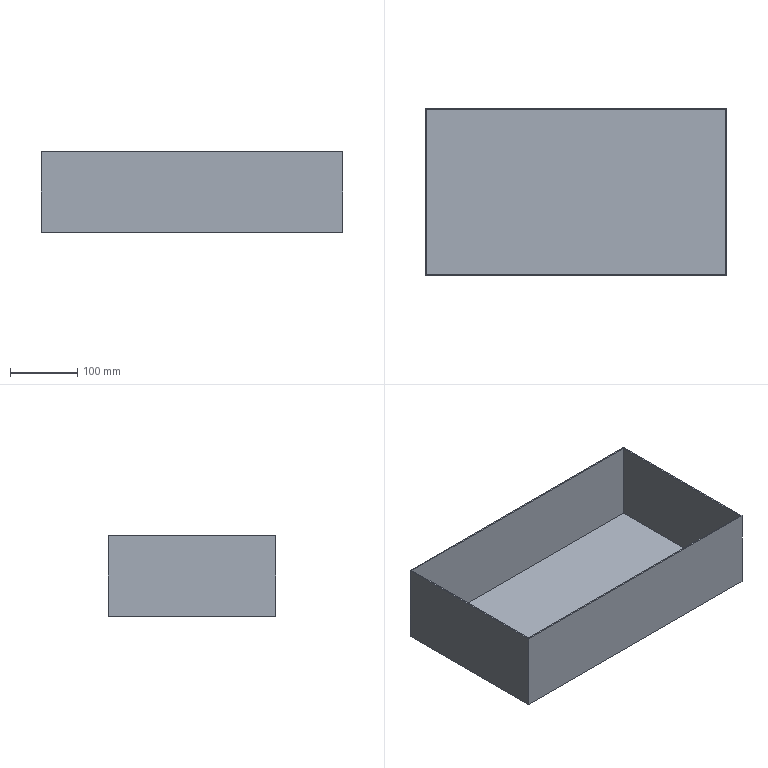Part | STEP file | NG parts material box | 1 solid | 11 faces | box 450 x 250 x 120 mm | volume 553512 mm3 | plane 11
STEP:
#1=CARTESIAN_POINT('',(0.,0.,0.));
#2=DIRECTION('',(0.,0.,1.));
#3=DIRECTION('',(1.,0.,0.));
#4=AXIS2_PLACEMENT_3D('',#1,#2,#3);
#5=CARTESIAN_POINT('',(-225.,-125.,0.));
#6=VERTEX_POINT('',#5);
#7=CARTESIAN_POINT('',(225.,-125.,0.));
#8=VERTEX_POINT('',#7);
#9=CARTESIAN_POINT('',(225.,-125.,0.));
#10=DIRECTION('',(1.,0.,0.));
#11=VECTOR('',#10,1.);
#12=LINE('',#9,#11);
#13=CARTESIAN_POINT('',(225.,-125.,0.));
#14=DIRECTION('',(0.,0.,1.));
#15=DIRECTION('',(1.,0.,0.));
#16=AXIS2_PLACEMENT_3D('',#13,#14,#15);
#17=PLANE('',#16);
#18=CARTESIAN_POINT('',(0.,0.));
#19=DIRECTION('',(1.,0.));
#20=VECTOR('',#19,1.);
#21=LINE('',#18,#20);
#22=(GEOMETRIC_REPRESENTATION_CONTEXT(2)PARAMETRIC_REPRESENTATION_CONTEXT()REPRESENTATION_CONTEXT('',''));
#23=DEFINITIONAL_REPRESENTATION('',(#21),#22);
#24=PCURVE('',#17,#23);
#25=CARTESIAN_POINT('',(-225.,-125.,120.));
#26=DIRECTION('',(0.,1.,0.));
#27=DIRECTION('',(0.,0.,1.));
#28=AXIS2_PLACEMENT_3D('',#25,#26,#27);
#29=PLANE('',#28);
#30=CARTESIAN_POINT('',(-120.,450.));
#31=DIRECTION('',(0.,1.));
#32=VECTOR('',#31,1.);
#33=LINE('',#30,#32);
#34=(GEOMETRIC_REPRESENTATION_CONTEXT(2)PARAMETRIC_REPRESENTATION_CONTEXT()REPRESENTATION_CONTEXT('',''));
#35=DEFINITIONAL_REPRESENTATION('',(#33),#34);
#36=PCURVE('',#29,#35);
#37=SURFACE_CURVE('',#12,(#24,#36),.PCURVE_S1.);
#38=EDGE_CURVE('',#6,#8,#37,.T.);
#39=ORIENTED_EDGE('',*,*,#38,.F.);
#40=CARTESIAN_POINT('',(-225.,125.,0.));
#41=VERTEX_POINT('',#40);
#42=CARTESIAN_POINT('',(-225.,-125.,0.));
#43=DIRECTION('',(0.,-1.,0.));
#44=VECTOR('',#43,1.);
#45=LINE('',#42,#44);
#46=CARTESIAN_POINT('',(-450.,0.));
#47=DIRECTION('',(0.,-1.));
#48=VECTOR('',#47,1.);
#49=LINE('',#46,#48);
#50=(GEOMETRIC_REPRESENTATION_CONTEXT(2)PARAMETRIC_REPRESENTATION_CONTEXT()REPRESENTATION_CONTEXT('',''));
#51=DEFINITIONAL_REPRESENTATION('',(#49),#50);
#52=PCURVE('',#17,#51);
#53=CARTESIAN_POINT('',(-225.,125.,120.));
#54=DIRECTION('',(1.,0.,0.));
#55=DIRECTION('',(0.,1.,0.));
#56=AXIS2_PLACEMENT_3D('',#53,#54,#55);
#57=PLANE('',#56);
#58=CARTESIAN_POINT('',(-250.,-120.));
#59=DIRECTION('',(-1.,0.));
#60=VECTOR('',#59,1.);
#61=LINE('',#58,#60);
#62=(GEOMETRIC_REPRESENTATION_CONTEXT(2)PARAMETRIC_REPRESENTATION_CONTEXT()REPRESENTATION_CONTEXT('',''));
#63=DEFINITIONAL_REPRESENTATION('',(#61),#62);
#64=PCURVE('',#57,#63);
#65=SURFACE_CURVE('',#45,(#52,#64),.PCURVE_S1.);
#66=EDGE_CURVE('',#41,#6,#65,.T.);
#67=ORIENTED_EDGE('',*,*,#66,.F.);
#68=CARTESIAN_POINT('',(225.,125.,0.));
#69=VERTEX_POINT('',#68);
#70=CARTESIAN_POINT('',(225.,125.,0.));
#71=DIRECTION('',(-1.,0.,0.));
#72=VECTOR('',#71,1.);
#73=LINE('',#70,#72);
#74=CARTESIAN_POINT('',(0.,250.));
#75=DIRECTION('',(-1.,0.));
#76=VECTOR('',#75,1.);
#77=LINE('',#74,#76);
#78=(GEOMETRIC_REPRESENTATION_CONTEXT(2)PARAMETRIC_REPRESENTATION_CONTEXT()REPRESENTATION_CONTEXT('',''));
#79=DEFINITIONAL_REPRESENTATION('',(#77),#78);
#80=PCURVE('',#17,#79);
#81=CARTESIAN_POINT('',(-225.,125.,120.));
#82=DIRECTION('',(0.,-1.,0.));
#83=DIRECTION('',(0.,0.,-1.));
#84=AXIS2_PLACEMENT_3D('',#81,#82,#83);
#85=PLANE('',#84);
#86=CARTESIAN_POINT('',(120.,450.));
#87=DIRECTION('',(0.,-1.));
#88=VECTOR('',#87,1.);
#89=LINE('',#86,#88);
#90=(GEOMETRIC_REPRESENTATION_CONTEXT(2)PARAMETRIC_REPRESENTATION_CONTEXT()REPRESENTATION_CONTEXT('',''));
#91=DEFINITIONAL_REPRESENTATION('',(#89),#90);
#92=PCURVE('',#85,#91);
#93=SURFACE_CURVE('',#73,(#80,#92),.PCURVE_S1.);
#94=EDGE_CURVE('',#69,#41,#93,.T.);
#95=ORIENTED_EDGE('',*,*,#94,.F.);
#96=CARTESIAN_POINT('',(225.,-125.,0.));
#97=DIRECTION('',(0.,1.,0.));
#98=VECTOR('',#97,1.);
#99=LINE('',#96,#98);
#100=CARTESIAN_POINT('',(0.,0.));
#101=DIRECTION('',(0.,1.));
#102=VECTOR('',#101,1.);
#103=LINE('',#100,#102);
#104=(GEOMETRIC_REPRESENTATION_CONTEXT(2)PARAMETRIC_REPRESENTATION_CONTEXT()REPRESENTATION_CONTEXT('',''));
#105=DEFINITIONAL_REPRESENTATION('',(#103),#104);
#106=PCURVE('',#17,#105);
#107=CARTESIAN_POINT('',(225.,125.,120.));
#108=DIRECTION('',(-1.,0.,0.));
#109=DIRECTION('',(0.,-1.,0.));
#110=AXIS2_PLACEMENT_3D('',#107,#108,#109);
#111=PLANE('',#110);
#112=CARTESIAN_POINT('',(250.,-120.));
#113=DIRECTION('',(-1.,0.));
#114=VECTOR('',#113,1.);
#115=LINE('',#112,#114);
#116=(GEOMETRIC_REPRESENTATION_CONTEXT(2)PARAMETRIC_REPRESENTATION_CONTEXT()REPRESENTATION_CONTEXT('',''));
#117=DEFINITIONAL_REPRESENTATION('',(#115),#116);
#118=PCURVE('',#111,#117);
#119=SURFACE_CURVE('',#99,(#106,#118),.PCURVE_S1.);
#120=EDGE_CURVE('',#8,#69,#119,.T.);
#121=ORIENTED_EDGE('',*,*,#120,.F.);
#122=EDGE_LOOP('',(#39,#67,#95,#121));
#123=FACE_BOUND('',#122,.T.);
#124=ADVANCED_FACE('',(#123),#17,.F.);
#125=CARTESIAN_POINT('',(225.,125.,120.));
#126=VERTEX_POINT('',#125);
#127=CARTESIAN_POINT('',(225.,125.,120.));
#128=DIRECTION('',(0.,0.,-1.));
#129=VECTOR('',#128,1.);
#130=LINE('',#127,#129);
#131=CARTESIAN_POINT('',(0.,0.));
#132=DIRECTION('',(0.,-1.));
#133=VECTOR('',#132,1.);
#134=LINE('',#131,#133);
#135=(GEOMETRIC_REPRESENTATION_CONTEXT(2)PARAMETRIC_REPRESENTATION_CONTEXT()REPRESENTATION_CONTEXT('',''));
#136=DEFINITIONAL_REPRESENTATION('',(#134),#135);
#137=PCURVE('',#111,#136);
#138=CARTESIAN_POINT('',(0.,450.));
#139=DIRECTION('',(1.,0.));
#140=VECTOR('',#139,1.);
#141=LINE('',#138,#140);
#142=(GEOMETRIC_REPRESENTATION_CONTEXT(2)PARAMETRIC_REPRESENTATION_CONTEXT()REPRESENTATION_CONTEXT('',''));
#143=DEFINITIONAL_REPRESENTATION('',(#141),#142);
#144=PCURVE('',#85,#143);
#145=SURFACE_CURVE('',#130,(#137,#144),.PCURVE_S1.);
#146=EDGE_CURVE('',#126,#69,#145,.T.);
#147=ORIENTED_EDGE('',*,*,#146,.F.);
#148=CARTESIAN_POINT('',(225.,-125.,120.));
#149=VERTEX_POINT('',#148);
#150=CARTESIAN_POINT('',(225.,125.,120.));
#151=DIRECTION('',(0.,1.,0.));
#152=VECTOR('',#151,1.);
#153=LINE('',#150,#152);
#154=CARTESIAN_POINT('',(0.,0.));
#155=DIRECTION('',(-1.,0.));
#156=VECTOR('',#155,1.);
#157=LINE('',#154,#156);
#158=(GEOMETRIC_REPRESENTATION_CONTEXT(2)PARAMETRIC_REPRESENTATION_CONTEXT()REPRESENTATION_CONTEXT('',''));
#159=DEFINITIONAL_REPRESENTATION('',(#157),#158);
#160=PCURVE('',#111,#159);
#161=CARTESIAN_POINT('',(225.,-125.,120.));
#162=DIRECTION('',(0.,0.,1.));
#163=DIRECTION('',(1.,0.,0.));
#164=AXIS2_PLACEMENT_3D('',#161,#162,#163);
#165=PLANE('',#164);
#166=CARTESIAN_POINT('',(0.,250.));
#167=DIRECTION('',(0.,1.));
#168=VECTOR('',#167,1.);
#169=LINE('',#166,#168);
#170=(GEOMETRIC_REPRESENTATION_CONTEXT(2)PARAMETRIC_REPRESENTATION_CONTEXT()REPRESENTATION_CONTEXT('',''));
#171=DEFINITIONAL_REPRESENTATION('',(#169),#170);
#172=PCURVE('',#165,#171);
#173=SURFACE_CURVE('',#153,(#160,#172),.PCURVE_S1.);
#174=EDGE_CURVE('',#149,#126,#173,.T.);
#175=ORIENTED_EDGE('',*,*,#174,.F.);
#176=CARTESIAN_POINT('',(225.,-125.,120.));
#177=DIRECTION('',(0.,0.,1.));
#178=VECTOR('',#177,1.);
#179=LINE('',#176,#178);
#180=CARTESIAN_POINT('',(250.,0.));
#181=DIRECTION('',(0.,1.));
#182=VECTOR('',#181,1.);
#183=LINE('',#180,#182);
#184=(GEOMETRIC_REPRESENTATION_CONTEXT(2)PARAMETRIC_REPRESENTATION_CONTEXT()REPRESENTATION_CONTEXT('',''));
#185=DEFINITIONAL_REPRESENTATION('',(#183),#184);
#186=PCURVE('',#111,#185);
#187=CARTESIAN_POINT('',(0.,450.));
#188=DIRECTION('',(1.,0.));
#189=VECTOR('',#188,1.);
#190=LINE('',#187,#189);
#191=(GEOMETRIC_REPRESENTATION_CONTEXT(2)PARAMETRIC_REPRESENTATION_CONTEXT()REPRESENTATION_CONTEXT('',''));
#192=DEFINITIONAL_REPRESENTATION('',(#190),#191);
#193=PCURVE('',#29,#192);
#194=SURFACE_CURVE('',#179,(#186,#193),.PCURVE_S1.);
#195=EDGE_CURVE('',#8,#149,#194,.T.);
#196=ORIENTED_EDGE('',*,*,#195,.F.);
#197=ORIENTED_EDGE('',*,*,#120,.T.);
#198=EDGE_LOOP('',(#147,#175,#196,#197));
#199=FACE_BOUND('',#198,.T.);
#200=ADVANCED_FACE('',(#199),#111,.F.);
#201=ORIENTED_EDGE('',*,*,#195,.T.);
#202=CARTESIAN_POINT('',(-225.,-125.,120.));
#203=VERTEX_POINT('',#202);
#204=CARTESIAN_POINT('',(-225.,-125.,120.));
#205=DIRECTION('',(1.,0.,0.));
#206=VECTOR('',#205,1.);
#207=LINE('',#204,#206);
#208=CARTESIAN_POINT('',(0.,0.));
#209=DIRECTION('',(0.,1.));
#210=VECTOR('',#209,1.);
#211=LINE('',#208,#210);
#212=(GEOMETRIC_REPRESENTATION_CONTEXT(2)PARAMETRIC_REPRESENTATION_CONTEXT()REPRESENTATION_CONTEXT('',''));
#213=DEFINITIONAL_REPRESENTATION('',(#211),#212);
#214=PCURVE('',#29,#213);
#215=CARTESIAN_POINT('',(-450.,0.));
#216=DIRECTION('',(1.,0.));
#217=VECTOR('',#216,1.);
#218=LINE('',#215,#217);
#219=(GEOMETRIC_REPRESENTATION_CONTEXT(2)PARAMETRIC_REPRESENTATION_CONTEXT()REPRESENTATION_CONTEXT('',''));
#220=DEFINITIONAL_REPRESENTATION('',(#218),#219);
#221=PCURVE('',#165,#220);
#222=SURFACE_CURVE('',#207,(#214,#221),.PCURVE_S1.);
#223=EDGE_CURVE('',#203,#149,#222,.T.);
#224=ORIENTED_EDGE('',*,*,#223,.F.);
#225=CARTESIAN_POINT('',(-225.,-125.,120.));
#226=DIRECTION('',(0.,0.,1.));
#227=VECTOR('',#226,1.);
#228=LINE('',#225,#227);
#229=CARTESIAN_POINT('',(0.,0.));
#230=DIRECTION('',(1.,0.));
#231=VECTOR('',#230,1.);
#232=LINE('',#229,#231);
#233=(GEOMETRIC_REPRESENTATION_CONTEXT(2)PARAMETRIC_REPRESENTATION_CONTEXT()REPRESENTATION_CONTEXT('',''));
#234=DEFINITIONAL_REPRESENTATION('',(#232),#233);
#235=PCURVE('',#29,#234);
#236=CARTESIAN_POINT('',(-250.,0.));
#237=DIRECTION('',(0.,1.));
#238=VECTOR('',#237,1.);
#239=LINE('',#236,#238);
#240=(GEOMETRIC_REPRESENTATION_CONTEXT(2)PARAMETRIC_REPRESENTATION_CONTEXT()REPRESENTATION_CONTEXT('',''));
#241=DEFINITIONAL_REPRESENTATION('',(#239),#240);
#242=PCURVE('',#57,#241);
#243=SURFACE_CURVE('',#228,(#235,#242),.PCURVE_S1.);
#244=EDGE_CURVE('',#6,#203,#243,.T.);
#245=ORIENTED_EDGE('',*,*,#244,.F.);
#246=ORIENTED_EDGE('',*,*,#38,.T.);
#247=EDGE_LOOP('',(#201,#224,#245,#246));
#248=FACE_BOUND('',#247,.T.);
#249=ADVANCED_FACE('',(#248),#29,.F.);
#250=ORIENTED_EDGE('',*,*,#244,.T.);
#251=CARTESIAN_POINT('',(-225.,125.,120.));
#252=VERTEX_POINT('',#251);
#253=CARTESIAN_POINT('',(-225.,125.,120.));
#254=DIRECTION('',(0.,-1.,0.));
#255=VECTOR('',#254,1.);
#256=LINE('',#253,#255);
#257=CARTESIAN_POINT('',(0.,0.));
#258=DIRECTION('',(-1.,0.));
#259=VECTOR('',#258,1.);
#260=LINE('',#257,#259);
#261=(GEOMETRIC_REPRESENTATION_CONTEXT(2)PARAMETRIC_REPRESENTATION_CONTEXT()REPRESENTATION_CONTEXT('',''));
#262=DEFINITIONAL_REPRESENTATION('',(#260),#261);
#263=PCURVE('',#57,#262);
#264=CARTESIAN_POINT('',(-450.,250.));
#265=DIRECTION('',(0.,-1.));
#266=VECTOR('',#265,1.);
#267=LINE('',#264,#266);
#268=(GEOMETRIC_REPRESENTATION_CONTEXT(2)PARAMETRIC_REPRESENTATION_CONTEXT()REPRESENTATION_CONTEXT('',''));
#269=DEFINITIONAL_REPRESENTATION('',(#267),#268);
#270=PCURVE('',#165,#269);
#271=SURFACE_CURVE('',#256,(#263,#270),.PCURVE_S1.);
#272=EDGE_CURVE('',#252,#203,#271,.T.);
#273=ORIENTED_EDGE('',*,*,#272,.F.);
#274=CARTESIAN_POINT('',(-225.,125.,120.));
#275=DIRECTION('',(0.,0.,1.));
#276=VECTOR('',#275,1.);
#277=LINE('',#274,#276);
#278=CARTESIAN_POINT('',(0.,0.));
#279=DIRECTION('',(0.,1.));
#280=VECTOR('',#279,1.);
#281=LINE('',#278,#280);
#282=(GEOMETRIC_REPRESENTATION_CONTEXT(2)PARAMETRIC_REPRESENTATION_CONTEXT()REPRESENTATION_CONTEXT('',''));
#283=DEFINITIONAL_REPRESENTATION('',(#281),#282);
#284=PCURVE('',#57,#283);
#285=CARTESIAN_POINT('',(0.,0.));
#286=DIRECTION('',(-1.,0.));
#287=VECTOR('',#286,1.);
#288=LINE('',#285,#287);
#289=(GEOMETRIC_REPRESENTATION_CONTEXT(2)PARAMETRIC_REPRESENTATION_CONTEXT()REPRESENTATION_CONTEXT('',''));
#290=DEFINITIONAL_REPRESENTATION('',(#288),#289);
#291=PCURVE('',#85,#290);
#292=SURFACE_CURVE('',#277,(#284,#291),.PCURVE_S1.);
#293=EDGE_CURVE('',#41,#252,#292,.T.);
#294=ORIENTED_EDGE('',*,*,#293,.F.);
#295=ORIENTED_EDGE('',*,*,#66,.T.);
#296=EDGE_LOOP('',(#250,#273,#294,#295));
#297=FACE_BOUND('',#296,.T.);
#298=ADVANCED_FACE('',(#297),#57,.F.);
#299=ORIENTED_EDGE('',*,*,#293,.T.);
#300=CARTESIAN_POINT('',(-225.,125.,120.));
#301=DIRECTION('',(-1.,0.,0.));
#302=VECTOR('',#301,1.);
#303=LINE('',#300,#302);
#304=CARTESIAN_POINT('',(0.,0.));
#305=DIRECTION('',(0.,-1.));
#306=VECTOR('',#305,1.);
#307=LINE('',#304,#306);
#308=(GEOMETRIC_REPRESENTATION_CONTEXT(2)PARAMETRIC_REPRESENTATION_CONTEXT()REPRESENTATION_CONTEXT('',''));
#309=DEFINITIONAL_REPRESENTATION('',(#307),#308);
#310=PCURVE('',#85,#309);
#311=CARTESIAN_POINT('',(-450.,250.));
#312=DIRECTION('',(-1.,0.));
#313=VECTOR('',#312,1.);
#314=LINE('',#311,#313);
#315=(GEOMETRIC_REPRESENTATION_CONTEXT(2)PARAMETRIC_REPRESENTATION_CONTEXT()REPRESENTATION_CONTEXT('',''));
#316=DEFINITIONAL_REPRESENTATION('',(#314),#315);
#317=PCURVE('',#165,#316);
#318=SURFACE_CURVE('',#303,(#310,#317),.PCURVE_S1.);
#319=EDGE_CURVE('',#126,#252,#318,.T.);
#320=ORIENTED_EDGE('',*,*,#319,.F.);
#321=ORIENTED_EDGE('',*,*,#146,.T.);
#322=ORIENTED_EDGE('',*,*,#94,.T.);
#323=EDGE_LOOP('',(#299,#320,#321,#322));
#324=FACE_BOUND('',#323,.T.);
#325=ADVANCED_FACE('',(#324),#85,.F.);
#326=ORIENTED_EDGE('',*,*,#272,.T.);
#327=ORIENTED_EDGE('',*,*,#223,.T.);
#328=ORIENTED_EDGE('',*,*,#174,.T.);
#329=ORIENTED_EDGE('',*,*,#319,.T.);
#330=EDGE_LOOP('',(#326,#327,#328,#329));
#331=FACE_BOUND('',#330,.T.);
#332=CARTESIAN_POINT('',(-223.,-123.,120.));
#333=VERTEX_POINT('',#332);
#334=CARTESIAN_POINT('',(-223.,123.,120.));
#335=VERTEX_POINT('',#334);
#336=CARTESIAN_POINT('',(-223.,-125.,120.));
#337=DIRECTION('',(0.,1.,0.));
#338=VECTOR('',#337,1.);
#339=LINE('',#336,#338);
#340=CARTESIAN_POINT('',(-448.,0.));
#341=DIRECTION('',(0.,1.));
#342=VECTOR('',#341,1.);
#343=LINE('',#340,#342);
#344=(GEOMETRIC_REPRESENTATION_CONTEXT(2)PARAMETRIC_REPRESENTATION_CONTEXT()REPRESENTATION_CONTEXT('',''));
#345=DEFINITIONAL_REPRESENTATION('',(#343),#344);
#346=PCURVE('',#165,#345);
#347=CARTESIAN_POINT('',(-223.,125.,120.));
#348=DIRECTION('',(1.,0.,0.));
#349=DIRECTION('',(0.,1.,0.));
#350=AXIS2_PLACEMENT_3D('',#347,#348,#349);
#351=PLANE('',#350);
#352=CARTESIAN_POINT('',(-250.,0.));
#353=DIRECTION('',(1.,0.));
#354=VECTOR('',#353,1.);
#355=LINE('',#352,#354);
#356=(GEOMETRIC_REPRESENTATION_CONTEXT(2)PARAMETRIC_REPRESENTATION_CONTEXT()REPRESENTATION_CONTEXT('',''));
#357=DEFINITIONAL_REPRESENTATION('',(#355),#356);
#358=PCURVE('',#351,#357);
#359=SURFACE_CURVE('',#339,(#346,#358),.PCURVE_S1.);
#360=EDGE_CURVE('',#333,#335,#359,.T.);
#361=ORIENTED_EDGE('',*,*,#360,.T.);
#362=CARTESIAN_POINT('',(223.,123.,120.));
#363=VERTEX_POINT('',#362);
#364=CARTESIAN_POINT('',(225.,123.,120.));
#365=DIRECTION('',(1.,0.,0.));
#366=VECTOR('',#365,1.);
#367=LINE('',#364,#366);
#368=CARTESIAN_POINT('',(0.,248.));
#369=DIRECTION('',(1.,0.));
#370=VECTOR('',#369,1.);
#371=LINE('',#368,#370);
#372=(GEOMETRIC_REPRESENTATION_CONTEXT(2)PARAMETRIC_REPRESENTATION_CONTEXT()REPRESENTATION_CONTEXT('',''));
#373=DEFINITIONAL_REPRESENTATION('',(#371),#372);
#374=PCURVE('',#165,#373);
#375=CARTESIAN_POINT('',(-225.,123.,120.));
#376=DIRECTION('',(0.,-1.,0.));
#377=DIRECTION('',(0.,0.,-1.));
#378=AXIS2_PLACEMENT_3D('',#375,#376,#377);
#379=PLANE('',#378);
#380=CARTESIAN_POINT('',(0.,450.));
#381=DIRECTION('',(0.,1.));
#382=VECTOR('',#381,1.);
#383=LINE('',#380,#382);
#384=(GEOMETRIC_REPRESENTATION_CONTEXT(2)PARAMETRIC_REPRESENTATION_CONTEXT()REPRESENTATION_CONTEXT('',''));
#385=DEFINITIONAL_REPRESENTATION('',(#383),#384);
#386=PCURVE('',#379,#385);
#387=SURFACE_CURVE('',#367,(#374,#386),.PCURVE_S1.);
#388=EDGE_CURVE('',#335,#363,#387,.T.);
#389=ORIENTED_EDGE('',*,*,#388,.T.);
#390=CARTESIAN_POINT('',(223.,-123.,120.));
#391=VERTEX_POINT('',#390);
#392=CARTESIAN_POINT('',(223.,-125.,120.));
#393=DIRECTION('',(0.,-1.,0.));
#394=VECTOR('',#393,1.);
#395=LINE('',#392,#394);
#396=CARTESIAN_POINT('',(-2.,0.));
#397=DIRECTION('',(0.,-1.));
#398=VECTOR('',#397,1.);
#399=LINE('',#396,#398);
#400=(GEOMETRIC_REPRESENTATION_CONTEXT(2)PARAMETRIC_REPRESENTATION_CONTEXT()REPRESENTATION_CONTEXT('',''));
#401=DEFINITIONAL_REPRESENTATION('',(#399),#400);
#402=PCURVE('',#165,#401);
#403=CARTESIAN_POINT('',(223.,125.,120.));
#404=DIRECTION('',(-1.,0.,0.));
#405=DIRECTION('',(0.,-1.,0.));
#406=AXIS2_PLACEMENT_3D('',#403,#404,#405);
#407=PLANE('',#406);
#408=CARTESIAN_POINT('',(250.,0.));
#409=DIRECTION('',(1.,0.));
#410=VECTOR('',#409,1.);
#411=LINE('',#408,#410);
#412=(GEOMETRIC_REPRESENTATION_CONTEXT(2)PARAMETRIC_REPRESENTATION_CONTEXT()REPRESENTATION_CONTEXT('',''));
#413=DEFINITIONAL_REPRESENTATION('',(#411),#412);
#414=PCURVE('',#407,#413);
#415=SURFACE_CURVE('',#395,(#402,#414),.PCURVE_S1.);
#416=EDGE_CURVE('',#363,#391,#415,.T.);
#417=ORIENTED_EDGE('',*,*,#416,.T.);
#418=CARTESIAN_POINT('',(225.,-123.,120.));
#419=DIRECTION('',(-1.,0.,0.));
#420=VECTOR('',#419,1.);
#421=LINE('',#418,#420);
#422=CARTESIAN_POINT('',(0.,2.));
#423=DIRECTION('',(-1.,0.));
#424=VECTOR('',#423,1.);
#425=LINE('',#422,#424);
#426=(GEOMETRIC_REPRESENTATION_CONTEXT(2)PARAMETRIC_REPRESENTATION_CONTEXT()REPRESENTATION_CONTEXT('',''));
#427=DEFINITIONAL_REPRESENTATION('',(#425),#426);
#428=PCURVE('',#165,#427);
#429=CARTESIAN_POINT('',(-225.,-123.,120.));
#430=DIRECTION('',(0.,1.,0.));
#431=DIRECTION('',(0.,0.,1.));
#432=AXIS2_PLACEMENT_3D('',#429,#430,#431);
#433=PLANE('',#432);
#434=CARTESIAN_POINT('',(0.,450.));
#435=DIRECTION('',(0.,-1.));
#436=VECTOR('',#435,1.);
#437=LINE('',#434,#436);
#438=(GEOMETRIC_REPRESENTATION_CONTEXT(2)PARAMETRIC_REPRESENTATION_CONTEXT()REPRESENTATION_CONTEXT('',''));
#439=DEFINITIONAL_REPRESENTATION('',(#437),#438);
#440=PCURVE('',#433,#439);
#441=SURFACE_CURVE('',#421,(#428,#440),.PCURVE_S1.);
#442=EDGE_CURVE('',#391,#333,#441,.T.);
#443=ORIENTED_EDGE('',*,*,#442,.T.);
#444=EDGE_LOOP('',(#361,#389,#417,#443));
#445=FACE_BOUND('',#444,.T.);
#446=ADVANCED_FACE('',(#331,#445),#165,.T.);
#447=ORIENTED_EDGE('',*,*,#388,.F.);
#448=CARTESIAN_POINT('',(-223.,123.,2.));
#449=VERTEX_POINT('',#448);
#450=CARTESIAN_POINT('',(-223.,123.,120.));
#451=DIRECTION('',(0.,0.,-1.));
#452=VECTOR('',#451,1.);
#453=LINE('',#450,#452);
#454=CARTESIAN_POINT('',(0.,2.));
#455=DIRECTION('',(1.,0.));
#456=VECTOR('',#455,1.);
#457=LINE('',#454,#456);
#458=(GEOMETRIC_REPRESENTATION_CONTEXT(2)PARAMETRIC_REPRESENTATION_CONTEXT()REPRESENTATION_CONTEXT('',''));
#459=DEFINITIONAL_REPRESENTATION('',(#457),#458);
#460=PCURVE('',#379,#459);
#461=CARTESIAN_POINT('',(-2.,0.));
#462=DIRECTION('',(0.,-1.));
#463=VECTOR('',#462,1.);
#464=LINE('',#461,#463);
#465=(GEOMETRIC_REPRESENTATION_CONTEXT(2)PARAMETRIC_REPRESENTATION_CONTEXT()REPRESENTATION_CONTEXT('',''));
#466=DEFINITIONAL_REPRESENTATION('',(#464),#465);
#467=PCURVE('',#351,#466);
#468=SURFACE_CURVE('',#453,(#460,#467),.PCURVE_S1.);
#469=EDGE_CURVE('',#335,#449,#468,.T.);
#470=ORIENTED_EDGE('',*,*,#469,.T.);
#471=CARTESIAN_POINT('',(223.,123.,2.));
#472=VERTEX_POINT('',#471);
#473=CARTESIAN_POINT('',(-225.,123.,2.));
#474=DIRECTION('',(1.,0.,0.));
#475=VECTOR('',#474,1.);
#476=LINE('',#473,#475);
#477=CARTESIAN_POINT('',(118.,0.));
#478=DIRECTION('',(0.,1.));
#479=VECTOR('',#478,1.);
#480=LINE('',#477,#479);
#481=(GEOMETRIC_REPRESENTATION_CONTEXT(2)PARAMETRIC_REPRESENTATION_CONTEXT()REPRESENTATION_CONTEXT('',''));
#482=DEFINITIONAL_REPRESENTATION('',(#480),#481);
#483=PCURVE('',#379,#482);
#484=CARTESIAN_POINT('',(225.,-125.,2.));
#485=DIRECTION('',(0.,0.,1.));
#486=DIRECTION('',(1.,0.,0.));
#487=AXIS2_PLACEMENT_3D('',#484,#485,#486);
#488=PLANE('',#487);
#489=CARTESIAN_POINT('',(-450.,248.));
#490=DIRECTION('',(1.,0.));
#491=VECTOR('',#490,1.);
#492=LINE('',#489,#491);
#493=(GEOMETRIC_REPRESENTATION_CONTEXT(2)PARAMETRIC_REPRESENTATION_CONTEXT()REPRESENTATION_CONTEXT('',''));
#494=DEFINITIONAL_REPRESENTATION('',(#492),#493);
#495=PCURVE('',#488,#494);
#496=SURFACE_CURVE('',#476,(#483,#495),.PCURVE_S1.);
#497=EDGE_CURVE('',#449,#472,#496,.T.);
#498=ORIENTED_EDGE('',*,*,#497,.T.);
#499=CARTESIAN_POINT('',(223.,123.,120.));
#500=DIRECTION('',(0.,0.,1.));
#501=VECTOR('',#500,1.);
#502=LINE('',#499,#501);
#503=CARTESIAN_POINT('',(0.,448.));
#504=DIRECTION('',(-1.,0.));
#505=VECTOR('',#504,1.);
#506=LINE('',#503,#505);
#507=(GEOMETRIC_REPRESENTATION_CONTEXT(2)PARAMETRIC_REPRESENTATION_CONTEXT()REPRESENTATION_CONTEXT('',''));
#508=DEFINITIONAL_REPRESENTATION('',(#506),#507);
#509=PCURVE('',#379,#508);
#510=CARTESIAN_POINT('',(2.,0.));
#511=DIRECTION('',(0.,1.));
#512=VECTOR('',#511,1.);
#513=LINE('',#510,#512);
#514=(GEOMETRIC_REPRESENTATION_CONTEXT(2)PARAMETRIC_REPRESENTATION_CONTEXT()REPRESENTATION_CONTEXT('',''));
#515=DEFINITIONAL_REPRESENTATION('',(#513),#514);
#516=PCURVE('',#407,#515);
#517=SURFACE_CURVE('',#502,(#509,#516),.PCURVE_S1.);
#518=EDGE_CURVE('',#472,#363,#517,.T.);
#519=ORIENTED_EDGE('',*,*,#518,.T.);
#520=EDGE_LOOP('',(#447,#470,#498,#519));
#521=FACE_BOUND('',#520,.T.);
#522=ADVANCED_FACE('',(#521),#379,.T.);
#523=ORIENTED_EDGE('',*,*,#360,.F.);
#524=CARTESIAN_POINT('',(-223.,-123.,2.));
#525=VERTEX_POINT('',#524);
#526=CARTESIAN_POINT('',(-223.,-123.,120.));
#527=DIRECTION('',(0.,0.,-1.));
#528=VECTOR('',#527,1.);
#529=LINE('',#526,#528);
#530=CARTESIAN_POINT('',(-248.,0.));
#531=DIRECTION('',(0.,-1.));
#532=VECTOR('',#531,1.);
#533=LINE('',#530,#532);
#534=(GEOMETRIC_REPRESENTATION_CONTEXT(2)PARAMETRIC_REPRESENTATION_CONTEXT()REPRESENTATION_CONTEXT('',''));
#535=DEFINITIONAL_REPRESENTATION('',(#533),#534);
#536=PCURVE('',#351,#535);
#537=CARTESIAN_POINT('',(0.,2.));
#538=DIRECTION('',(-1.,0.));
#539=VECTOR('',#538,1.);
#540=LINE('',#537,#539);
#541=(GEOMETRIC_REPRESENTATION_CONTEXT(2)PARAMETRIC_REPRESENTATION_CONTEXT()REPRESENTATION_CONTEXT('',''));
#542=DEFINITIONAL_REPRESENTATION('',(#540),#541);
#543=PCURVE('',#433,#542);
#544=SURFACE_CURVE('',#529,(#536,#543),.PCURVE_S1.);
#545=EDGE_CURVE('',#333,#525,#544,.T.);
#546=ORIENTED_EDGE('',*,*,#545,.T.);
#547=CARTESIAN_POINT('',(-223.,125.,2.));
#548=DIRECTION('',(0.,1.,0.));
#549=VECTOR('',#548,1.);
#550=LINE('',#547,#549);
#551=CARTESIAN_POINT('',(0.,-118.));
#552=DIRECTION('',(1.,0.));
#553=VECTOR('',#552,1.);
#554=LINE('',#551,#553);
#555=(GEOMETRIC_REPRESENTATION_CONTEXT(2)PARAMETRIC_REPRESENTATION_CONTEXT()REPRESENTATION_CONTEXT('',''));
#556=DEFINITIONAL_REPRESENTATION('',(#554),#555);
#557=PCURVE('',#351,#556);
#558=CARTESIAN_POINT('',(-448.,250.));
#559=DIRECTION('',(0.,1.));
#560=VECTOR('',#559,1.);
#561=LINE('',#558,#560);
#562=(GEOMETRIC_REPRESENTATION_CONTEXT(2)PARAMETRIC_REPRESENTATION_CONTEXT()REPRESENTATION_CONTEXT('',''));
#563=DEFINITIONAL_REPRESENTATION('',(#561),#562);
#564=PCURVE('',#488,#563);
#565=SURFACE_CURVE('',#550,(#557,#564),.PCURVE_S1.);
#566=EDGE_CURVE('',#525,#449,#565,.T.);
#567=ORIENTED_EDGE('',*,*,#566,.T.);
#568=ORIENTED_EDGE('',*,*,#469,.F.);
#569=EDGE_LOOP('',(#523,#546,#567,#568));
#570=FACE_BOUND('',#569,.T.);
#571=ADVANCED_FACE('',(#570),#351,.T.);
#572=ORIENTED_EDGE('',*,*,#442,.F.);
#573=CARTESIAN_POINT('',(223.,-123.,2.));
#574=VERTEX_POINT('',#573);
#575=CARTESIAN_POINT('',(223.,-123.,120.));
#576=DIRECTION('',(0.,0.,-1.));
#577=VECTOR('',#576,1.);
#578=LINE('',#575,#577);
#579=CARTESIAN_POINT('',(0.,448.));
#580=DIRECTION('',(-1.,0.));
#581=VECTOR('',#580,1.);
#582=LINE('',#579,#581);
#583=(GEOMETRIC_REPRESENTATION_CONTEXT(2)PARAMETRIC_REPRESENTATION_CONTEXT()REPRESENTATION_CONTEXT('',''));
#584=DEFINITIONAL_REPRESENTATION('',(#582),#583);
#585=PCURVE('',#433,#584);
#586=CARTESIAN_POINT('',(248.,0.));
#587=DIRECTION('',(0.,-1.));
#588=VECTOR('',#587,1.);
#589=LINE('',#586,#588);
#590=(GEOMETRIC_REPRESENTATION_CONTEXT(2)PARAMETRIC_REPRESENTATION_CONTEXT()REPRESENTATION_CONTEXT('',''));
#591=DEFINITIONAL_REPRESENTATION('',(#589),#590);
#592=PCURVE('',#407,#591);
#593=SURFACE_CURVE('',#578,(#585,#592),.PCURVE_S1.);
#594=EDGE_CURVE('',#391,#574,#593,.T.);
#595=ORIENTED_EDGE('',*,*,#594,.T.);
#596=CARTESIAN_POINT('',(-225.,-123.,2.));
#597=DIRECTION('',(-1.,0.,0.));
#598=VECTOR('',#597,1.);
#599=LINE('',#596,#598);
#600=CARTESIAN_POINT('',(-118.,0.));
#601=DIRECTION('',(0.,-1.));
#602=VECTOR('',#601,1.);
#603=LINE('',#600,#602);
#604=(GEOMETRIC_REPRESENTATION_CONTEXT(2)PARAMETRIC_REPRESENTATION_CONTEXT()REPRESENTATION_CONTEXT('',''));
#605=DEFINITIONAL_REPRESENTATION('',(#603),#604);
#606=PCURVE('',#433,#605);
#607=CARTESIAN_POINT('',(-450.,2.));
#608=DIRECTION('',(-1.,0.));
#609=VECTOR('',#608,1.);
#610=LINE('',#607,#609);
#611=(GEOMETRIC_REPRESENTATION_CONTEXT(2)PARAMETRIC_REPRESENTATION_CONTEXT()REPRESENTATION_CONTEXT('',''));
#612=DEFINITIONAL_REPRESENTATION('',(#610),#611);
#613=PCURVE('',#488,#612);
#614=SURFACE_CURVE('',#599,(#606,#613),.PCURVE_S1.);
#615=EDGE_CURVE('',#574,#525,#614,.T.);
#616=ORIENTED_EDGE('',*,*,#615,.T.);
#617=ORIENTED_EDGE('',*,*,#545,.F.);
#618=EDGE_LOOP('',(#572,#595,#616,#617));
#619=FACE_BOUND('',#618,.T.);
#620=ADVANCED_FACE('',(#619),#433,.T.);
#621=ORIENTED_EDGE('',*,*,#416,.F.);
#622=ORIENTED_EDGE('',*,*,#518,.F.);
#623=CARTESIAN_POINT('',(223.,125.,2.));
#624=DIRECTION('',(0.,-1.,0.));
#625=VECTOR('',#624,1.);
#626=LINE('',#623,#625);
#627=CARTESIAN_POINT('',(0.,-118.));
#628=DIRECTION('',(1.,0.));
#629=VECTOR('',#628,1.);
#630=LINE('',#627,#629);
#631=(GEOMETRIC_REPRESENTATION_CONTEXT(2)PARAMETRIC_REPRESENTATION_CONTEXT()REPRESENTATION_CONTEXT('',''));
#632=DEFINITIONAL_REPRESENTATION('',(#630),#631);
#633=PCURVE('',#407,#632);
#634=CARTESIAN_POINT('',(-2.,250.));
#635=DIRECTION('',(0.,-1.));
#636=VECTOR('',#635,1.);
#637=LINE('',#634,#636);
#638=(GEOMETRIC_REPRESENTATION_CONTEXT(2)PARAMETRIC_REPRESENTATION_CONTEXT()REPRESENTATION_CONTEXT('',''));
#639=DEFINITIONAL_REPRESENTATION('',(#637),#638);
#640=PCURVE('',#488,#639);
#641=SURFACE_CURVE('',#626,(#633,#640),.PCURVE_S1.);
#642=EDGE_CURVE('',#472,#574,#641,.T.);
#643=ORIENTED_EDGE('',*,*,#642,.T.);
#644=ORIENTED_EDGE('',*,*,#594,.F.);
#645=EDGE_LOOP('',(#621,#622,#643,#644));
#646=FACE_BOUND('',#645,.T.);
#647=ADVANCED_FACE('',(#646),#407,.T.);
#648=ORIENTED_EDGE('',*,*,#566,.F.);
#649=ORIENTED_EDGE('',*,*,#615,.F.);
#650=ORIENTED_EDGE('',*,*,#642,.F.);
#651=ORIENTED_EDGE('',*,*,#497,.F.);
#652=EDGE_LOOP('',(#648,#649,#650,#651));
#653=FACE_BOUND('',#652,.T.);
#654=ADVANCED_FACE('',(#653),#488,.T.);
#655=CLOSED_SHELL('',(#124,#200,#249,#298,#325,#446,#522,#571,#620,#647,#654));
#656=MANIFOLD_SOLID_BREP('',#655);
#657=(LENGTH_UNIT()NAMED_UNIT(*)SI_UNIT(.MILLI.,.METRE.));
#658=UNCERTAINTY_MEASURE_WITH_UNIT(LENGTH_MEASURE(0.0000001),#657,'','');
#659=(NAMED_UNIT(*)PLANE_ANGLE_UNIT()SI_UNIT($,.RADIAN.));
#660=(NAMED_UNIT(*)SI_UNIT($,.STERADIAN.)SOLID_ANGLE_UNIT());
#661=(GEOMETRIC_REPRESENTATION_CONTEXT(3)GLOBAL_UNCERTAINTY_ASSIGNED_CONTEXT((#658))GLOBAL_UNIT_ASSIGNED_CONTEXT((#657,#659,#660))REPRESENTATION_CONTEXT('',''));
#662=ADVANCED_BREP_SHAPE_REPRESENTATION('',(#4,#656),#661);